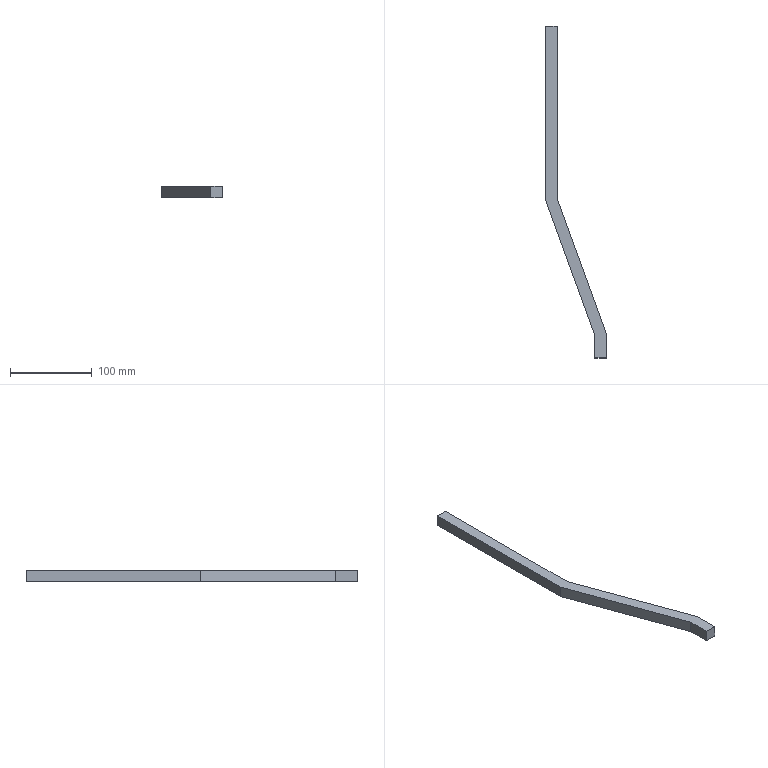Part | NX | features solid 2 | 1 solid | 10 faces | box 74 x 405 x 14 mm | volume 81454 mm3 | plane 10
STEP:
#1=CARTESIAN_POINT('',(300.,335.,-5.));
#2=VERTEX_POINT('',#1);
#3=CARTESIAN_POINT('',(300.,122.355,-5.));
#4=VERTEX_POINT('',#3);
#5=CARTESIAN_POINT('',(300.,150.,-5.));
#6=DIRECTION('',(0.,-1.,0.));
#7=VECTOR('',#6,1000.);
#8=LINE('',#5,#7);
#9=EDGE_CURVE('',#2,#4,#8,.T.);
#10=ORIENTED_EDGE('',*,*,#9,.T.);
#11=CARTESIAN_POINT('',(300.,122.355,9.));
#12=VERTEX_POINT('',#11);
#13=CARTESIAN_POINT('',(300.,122.355,9.));
#14=DIRECTION('',(0.,0.,-1.));
#15=VECTOR('',#14,1000.);
#16=LINE('',#13,#15);
#17=EDGE_CURVE('',#12,#4,#16,.T.);
#18=ORIENTED_EDGE('',*,*,#17,.F.);
#19=CARTESIAN_POINT('',(300.,335.,9.));
#20=VERTEX_POINT('',#19);
#21=CARTESIAN_POINT('',(300.,245.,9.));
#22=DIRECTION('',(0.,-1.,0.));
#23=VECTOR('',#22,1000.);
#24=LINE('',#21,#23);
#25=EDGE_CURVE('',#20,#12,#24,.T.);
#26=ORIENTED_EDGE('',*,*,#25,.F.);
#27=CARTESIAN_POINT('',(300.,335.,9.));
#28=DIRECTION('',(0.,0.,-1.));
#29=VECTOR('',#28,1000.);
#30=LINE('',#27,#29);
#31=EDGE_CURVE('',#20,#2,#30,.T.);
#32=ORIENTED_EDGE('',*,*,#31,.T.);
#33=EDGE_LOOP('',(#10,#18,#26,#32));
#34=FACE_BOUND('',#33,.T.);
#35=CARTESIAN_POINT('',(300.,150.,9.));
#36=DIRECTION('',(1.,0.,0.));
#37=DIRECTION('',(0.,1.,0.));
#38=AXIS2_PLACEMENT_3D('',#35,#36,#37);
#39=PLANE('',#38);
#40=ADVANCED_FACE('',(#34),#39,.F.);
#41=CARTESIAN_POINT('',(360.,-42.494,-5.));
#42=VERTEX_POINT('',#41);
#43=CARTESIAN_POINT('',(344.534,0.,-5.));
#44=DIRECTION('',(0.342,-0.9397,0.));
#45=VECTOR('',#44,1000.);
#46=LINE('',#43,#45);
#47=EDGE_CURVE('',#4,#42,#46,.T.);
#48=ORIENTED_EDGE('',*,*,#47,.T.);
#49=CARTESIAN_POINT('',(360.,-42.494,9.));
#50=VERTEX_POINT('',#49);
#51=CARTESIAN_POINT('',(360.,-42.494,9.));
#52=DIRECTION('',(0.,0.,-1.));
#53=VECTOR('',#52,1000.);
#54=LINE('',#51,#53);
#55=EDGE_CURVE('',#50,#42,#54,.T.);
#56=ORIENTED_EDGE('',*,*,#55,.F.);
#57=CARTESIAN_POINT('',(300.,122.355,9.));
#58=DIRECTION('',(0.342,-0.9397,0.));
#59=VECTOR('',#58,1000.);
#60=LINE('',#57,#59);
#61=EDGE_CURVE('',#12,#50,#60,.T.);
#62=ORIENTED_EDGE('',*,*,#61,.F.);
#63=ORIENTED_EDGE('',*,*,#17,.T.);
#64=EDGE_LOOP('',(#48,#56,#62,#63));
#65=FACE_BOUND('',#64,.T.);
#66=CARTESIAN_POINT('',(344.534,0.,9.));
#67=DIRECTION('',(0.9397,0.342,0.));
#68=DIRECTION('',(-0.342,0.9397,0.));
#69=AXIS2_PLACEMENT_3D('',#66,#67,#68);
#70=PLANE('',#69);
#71=ADVANCED_FACE('',(#65),#70,.F.);
#72=CARTESIAN_POINT('',(360.,-70.,-5.));
#73=VERTEX_POINT('',#72);
#74=CARTESIAN_POINT('',(360.,-42.494,-5.));
#75=DIRECTION('',(0.,-1.,0.));
#76=VECTOR('',#75,1000.);
#77=LINE('',#74,#76);
#78=EDGE_CURVE('',#42,#73,#77,.T.);
#79=ORIENTED_EDGE('',*,*,#78,.T.);
#80=CARTESIAN_POINT('',(360.,-70.,9.));
#81=VERTEX_POINT('',#80);
#82=CARTESIAN_POINT('',(360.,-70.,9.));
#83=DIRECTION('',(0.,0.,-1.));
#84=VECTOR('',#83,1000.);
#85=LINE('',#82,#84);
#86=EDGE_CURVE('',#81,#73,#85,.T.);
#87=ORIENTED_EDGE('',*,*,#86,.F.);
#88=CARTESIAN_POINT('',(360.,-42.494,9.));
#89=DIRECTION('',(0.,-1.,0.));
#90=VECTOR('',#89,1000.);
#91=LINE('',#88,#90);
#92=EDGE_CURVE('',#50,#81,#91,.T.);
#93=ORIENTED_EDGE('',*,*,#92,.F.);
#94=ORIENTED_EDGE('',*,*,#55,.T.);
#95=EDGE_LOOP('',(#79,#87,#93,#94));
#96=FACE_BOUND('',#95,.T.);
#97=CARTESIAN_POINT('',(360.,-42.494,9.));
#98=DIRECTION('',(1.,0.,0.));
#99=DIRECTION('',(0.,0.,-1.));
#100=AXIS2_PLACEMENT_3D('',#97,#98,#99);
#101=PLANE('',#100);
#102=ADVANCED_FACE('',(#96),#101,.F.);
#103=CARTESIAN_POINT('',(374.,-70.,-5.));
#104=VERTEX_POINT('',#103);
#105=CARTESIAN_POINT('',(360.,-70.,-5.));
#106=DIRECTION('',(1.,0.,0.));
#107=VECTOR('',#106,1000.);
#108=LINE('',#105,#107);
#109=EDGE_CURVE('',#73,#104,#108,.T.);
#110=ORIENTED_EDGE('',*,*,#109,.T.);
#111=CARTESIAN_POINT('',(374.,-70.,9.));
#112=VERTEX_POINT('',#111);
#113=CARTESIAN_POINT('',(374.,-70.,9.));
#114=DIRECTION('',(0.,0.,-1.));
#115=VECTOR('',#114,1000.);
#116=LINE('',#113,#115);
#117=EDGE_CURVE('',#112,#104,#116,.T.);
#118=ORIENTED_EDGE('',*,*,#117,.F.);
#119=CARTESIAN_POINT('',(360.,-70.,9.));
#120=DIRECTION('',(1.,0.,0.));
#121=VECTOR('',#120,1000.);
#122=LINE('',#119,#121);
#123=EDGE_CURVE('',#81,#112,#122,.T.);
#124=ORIENTED_EDGE('',*,*,#123,.F.);
#125=ORIENTED_EDGE('',*,*,#86,.T.);
#126=EDGE_LOOP('',(#110,#118,#124,#125));
#127=FACE_BOUND('',#126,.T.);
#128=CARTESIAN_POINT('',(360.,-70.,9.));
#129=DIRECTION('',(0.,1.,0.));
#130=DIRECTION('',(0.,0.,1.));
#131=AXIS2_PLACEMENT_3D('',#128,#129,#130);
#132=PLANE('',#131);
#133=ADVANCED_FACE('',(#127),#132,.F.);
#134=CARTESIAN_POINT('',(374.,-40.025,-5.));
#135=VERTEX_POINT('',#134);
#136=CARTESIAN_POINT('',(374.,-40.025,-5.));
#137=DIRECTION('',(0.,-1.,0.));
#138=VECTOR('',#137,1000.);
#139=LINE('',#136,#138);
#140=EDGE_CURVE('',#135,#104,#139,.T.);
#141=ORIENTED_EDGE('',*,*,#140,.F.);
#142=CARTESIAN_POINT('',(374.,-40.025,9.));
#143=VERTEX_POINT('',#142);
#144=CARTESIAN_POINT('',(374.,-40.025,9.));
#145=DIRECTION('',(0.,0.,-1.));
#146=VECTOR('',#145,1000.);
#147=LINE('',#144,#146);
#148=EDGE_CURVE('',#143,#135,#147,.T.);
#149=ORIENTED_EDGE('',*,*,#148,.F.);
#150=CARTESIAN_POINT('',(374.,-40.025,9.));
#151=DIRECTION('',(0.,-1.,0.));
#152=VECTOR('',#151,1000.);
#153=LINE('',#150,#152);
#154=EDGE_CURVE('',#143,#112,#153,.T.);
#155=ORIENTED_EDGE('',*,*,#154,.T.);
#156=ORIENTED_EDGE('',*,*,#117,.T.);
#157=EDGE_LOOP('',(#141,#149,#155,#156));
#158=FACE_BOUND('',#157,.T.);
#159=CARTESIAN_POINT('',(374.,-40.025,9.));
#160=DIRECTION('',(1.,0.,0.));
#161=DIRECTION('',(0.,0.,-1.));
#162=AXIS2_PLACEMENT_3D('',#159,#160,#161);
#163=PLANE('',#162);
#164=ADVANCED_FACE('',(#158),#163,.T.);
#165=CARTESIAN_POINT('',(314.,124.824,-5.));
#166=VERTEX_POINT('',#165);
#167=CARTESIAN_POINT('',(314.,124.824,-5.));
#168=DIRECTION('',(0.342,-0.9397,0.));
#169=VECTOR('',#168,1000.);
#170=LINE('',#167,#169);
#171=EDGE_CURVE('',#166,#135,#170,.T.);
#172=ORIENTED_EDGE('',*,*,#171,.F.);
#173=CARTESIAN_POINT('',(314.,124.824,9.));
#174=VERTEX_POINT('',#173);
#175=CARTESIAN_POINT('',(314.,124.824,9.));
#176=DIRECTION('',(0.,0.,-1.));
#177=VECTOR('',#176,1000.);
#178=LINE('',#175,#177);
#179=EDGE_CURVE('',#174,#166,#178,.T.);
#180=ORIENTED_EDGE('',*,*,#179,.F.);
#181=CARTESIAN_POINT('',(359.557,-0.342,9.));
#182=DIRECTION('',(0.342,-0.9397,0.));
#183=VECTOR('',#182,1000.);
#184=LINE('',#181,#183);
#185=EDGE_CURVE('',#174,#143,#184,.T.);
#186=ORIENTED_EDGE('',*,*,#185,.T.);
#187=ORIENTED_EDGE('',*,*,#148,.T.);
#188=EDGE_LOOP('',(#172,#180,#186,#187));
#189=FACE_BOUND('',#188,.T.);
#190=CARTESIAN_POINT('',(314.,124.824,9.));
#191=DIRECTION('',(0.9397,0.342,0.));
#192=DIRECTION('',(-0.342,0.9397,0.));
#193=AXIS2_PLACEMENT_3D('',#190,#191,#192);
#194=PLANE('',#193);
#195=ADVANCED_FACE('',(#189),#194,.T.);
#196=CARTESIAN_POINT('',(314.,335.,-5.));
#197=VERTEX_POINT('',#196);
#198=CARTESIAN_POINT('',(314.,335.,-5.));
#199=DIRECTION('',(0.,-1.,0.));
#200=VECTOR('',#199,1000.);
#201=LINE('',#198,#200);
#202=EDGE_CURVE('',#197,#166,#201,.T.);
#203=ORIENTED_EDGE('',*,*,#202,.F.);
#204=CARTESIAN_POINT('',(314.,335.,9.));
#205=VERTEX_POINT('',#204);
#206=CARTESIAN_POINT('',(314.,335.,9.));
#207=DIRECTION('',(0.,0.,-1.));
#208=VECTOR('',#207,1000.);
#209=LINE('',#206,#208);
#210=EDGE_CURVE('',#205,#197,#209,.T.);
#211=ORIENTED_EDGE('',*,*,#210,.F.);
#212=CARTESIAN_POINT('',(314.,150.,9.));
#213=DIRECTION('',(0.,-1.,0.));
#214=VECTOR('',#213,1000.);
#215=LINE('',#212,#214);
#216=EDGE_CURVE('',#205,#174,#215,.T.);
#217=ORIENTED_EDGE('',*,*,#216,.T.);
#218=ORIENTED_EDGE('',*,*,#179,.T.);
#219=EDGE_LOOP('',(#203,#211,#217,#218));
#220=FACE_BOUND('',#219,.T.);
#221=CARTESIAN_POINT('',(314.,335.,9.));
#222=DIRECTION('',(1.,0.,0.));
#223=DIRECTION('',(0.,0.,-1.));
#224=AXIS2_PLACEMENT_3D('',#221,#222,#223);
#225=PLANE('',#224);
#226=ADVANCED_FACE('',(#220),#225,.T.);
#227=CARTESIAN_POINT('',(314.,335.,-5.));
#228=DIRECTION('',(-1.,0.,0.));
#229=VECTOR('',#228,1000.);
#230=LINE('',#227,#229);
#231=EDGE_CURVE('',#197,#2,#230,.T.);
#232=ORIENTED_EDGE('',*,*,#231,.T.);
#233=ORIENTED_EDGE('',*,*,#31,.F.);
#234=CARTESIAN_POINT('',(314.,335.,9.));
#235=DIRECTION('',(-1.,0.,0.));
#236=VECTOR('',#235,1000.);
#237=LINE('',#234,#236);
#238=EDGE_CURVE('',#205,#20,#237,.T.);
#239=ORIENTED_EDGE('',*,*,#238,.F.);
#240=ORIENTED_EDGE('',*,*,#210,.T.);
#241=EDGE_LOOP('',(#232,#233,#239,#240));
#242=FACE_BOUND('',#241,.T.);
#243=CARTESIAN_POINT('',(314.,335.,9.));
#244=DIRECTION('',(0.,-1.,0.));
#245=DIRECTION('',(0.,0.,-1.));
#246=AXIS2_PLACEMENT_3D('',#243,#244,#245);
#247=PLANE('',#246);
#248=ADVANCED_FACE('',(#242),#247,.F.);
#249=ORIENTED_EDGE('',*,*,#238,.T.);
#250=ORIENTED_EDGE('',*,*,#25,.T.);
#251=ORIENTED_EDGE('',*,*,#61,.T.);
#252=ORIENTED_EDGE('',*,*,#92,.T.);
#253=ORIENTED_EDGE('',*,*,#123,.T.);
#254=ORIENTED_EDGE('',*,*,#154,.F.);
#255=ORIENTED_EDGE('',*,*,#185,.F.);
#256=ORIENTED_EDGE('',*,*,#216,.F.);
#257=EDGE_LOOP('',(#249,#250,#251,#252,#253,#254,#255,#256));
#258=FACE_BOUND('',#257,.T.);
#259=CARTESIAN_POINT('',(300.,-70.,9.));
#260=DIRECTION('',(0.,0.,1.));
#261=DIRECTION('',(1.,0.,0.));
#262=AXIS2_PLACEMENT_3D('',#259,#260,#261);
#263=PLANE('',#262);
#264=ADVANCED_FACE('',(#258),#263,.T.);
#265=ORIENTED_EDGE('',*,*,#9,.F.);
#266=ORIENTED_EDGE('',*,*,#231,.F.);
#267=ORIENTED_EDGE('',*,*,#202,.T.);
#268=ORIENTED_EDGE('',*,*,#171,.T.);
#269=ORIENTED_EDGE('',*,*,#140,.T.);
#270=ORIENTED_EDGE('',*,*,#109,.F.);
#271=ORIENTED_EDGE('',*,*,#78,.F.);
#272=ORIENTED_EDGE('',*,*,#47,.F.);
#273=EDGE_LOOP('',(#265,#266,#267,#268,#269,#270,#271,#272));
#274=FACE_BOUND('',#273,.T.);
#275=CARTESIAN_POINT('',(300.,-70.,-5.));
#276=DIRECTION('',(0.,0.,1.));
#277=DIRECTION('',(1.,0.,0.));
#278=AXIS2_PLACEMENT_3D('',#275,#276,#277);
#279=PLANE('',#278);
#280=ADVANCED_FACE('',(#274),#279,.F.);
#281=CLOSED_SHELL('',(#40,#71,#102,#133,#164,#195,#226,#248,#264,#280));
#282=MANIFOLD_SOLID_BREP('',#281);
#283=(LENGTH_UNIT()NAMED_UNIT(*)SI_UNIT(.MILLI.,.METRE.));
#284=UNCERTAINTY_MEASURE_WITH_UNIT(LENGTH_MEASURE(0.00001),#283,'','');
#285=(NAMED_UNIT(*)PLANE_ANGLE_UNIT()SI_UNIT($,.RADIAN.));
#286=(NAMED_UNIT(*)SI_UNIT($,.STERADIAN.)SOLID_ANGLE_UNIT());
#287=(GEOMETRIC_REPRESENTATION_CONTEXT(3)GLOBAL_UNCERTAINTY_ASSIGNED_CONTEXT((#284))GLOBAL_UNIT_ASSIGNED_CONTEXT((#283,#285,#286))REPRESENTATION_CONTEXT('',''));
#288=ADVANCED_BREP_SHAPE_REPRESENTATION('',(#282),#287);